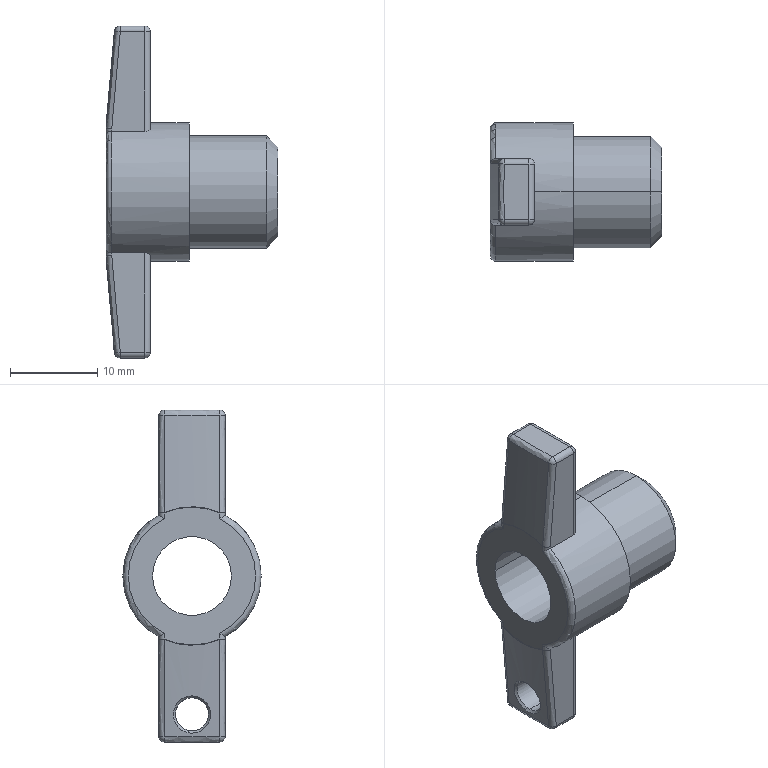Part | STEP file | 4-20.sldasm-Part-62 | 1 solid | 63 faces | box 19.685 x 15.875 x 38.1 mm | volume 2641 mm3 | cylinder 22 | spline 12 | sphere 12 | plane 11 | cone 4 | torus 2 | commonest cylinder face diameters 1.27 x14 3.81 x2 9.047 x2 12.857 x2 15.875 x2